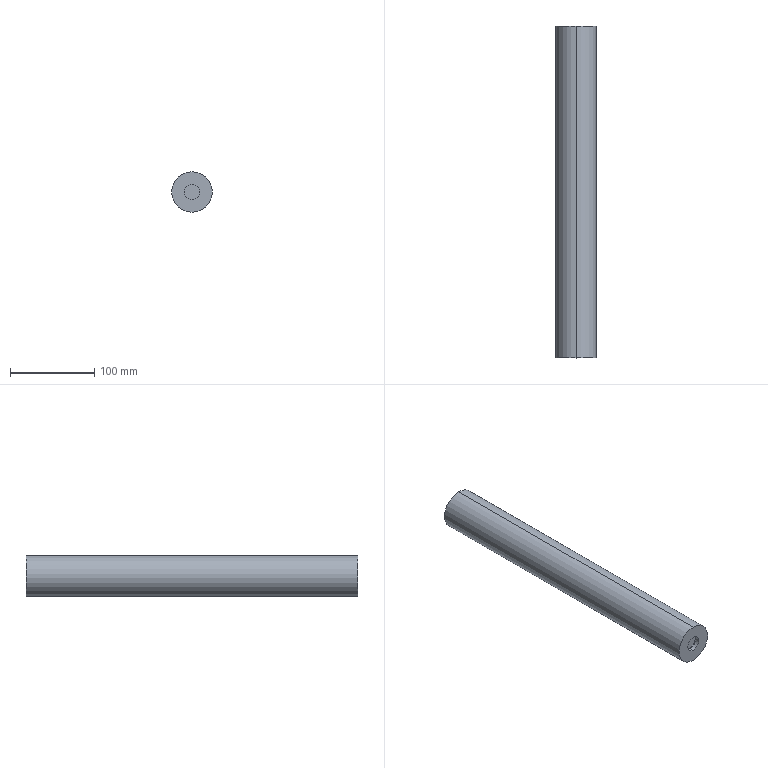Part | SolidWorks | features 3DProfileFeature 1, HoleWzd 1, Revolution 1 | 1 solid | 14 faces | box 48 x 395 x 48 mm | volume 696230 mm3 | cylinder 8 | plane 4 | cone 2 | commonest cylinder face diameters 18.5 x2 23 x2 25 x2 48 x2
STEP:
#1=CARTESIAN_POINT('',(0.,365.,-12.5));
#2=VERTEX_POINT('',#1);
#3=CARTESIAN_POINT('',(0.,365.,12.5));
#4=VERTEX_POINT('',#3);
#5=CARTESIAN_POINT('',(0.,365.,0.));
#6=DIRECTION('',(0.,1.,0.));
#7=DIRECTION('',(0.,0.,1.));
#8=AXIS2_PLACEMENT_3D('',#5,#6,#7);
#9=CIRCLE('',#8,12.5);
#10=EDGE_CURVE('',#2,#4,#9,.T.);
#11=ORIENTED_EDGE('',*,*,#10,.F.);
#12=CARTESIAN_POINT('',(0.,395.,-12.5));
#13=VERTEX_POINT('',#12);
#14=CARTESIAN_POINT('',(0.,395.,-12.5));
#15=DIRECTION('',(0.,1.,0.));
#16=VECTOR('',#15,1000.);
#17=LINE('',#14,#16);
#18=EDGE_CURVE('',#2,#13,#17,.T.);
#19=ORIENTED_EDGE('',*,*,#18,.T.);
#20=CARTESIAN_POINT('',(0.,395.,12.5));
#21=VERTEX_POINT('',#20);
#22=CARTESIAN_POINT('',(0.,395.,0.));
#23=DIRECTION('',(0.,1.,0.));
#24=DIRECTION('',(0.,0.,1.));
#25=AXIS2_PLACEMENT_3D('',#22,#23,#24);
#26=CIRCLE('',#25,12.5);
#27=EDGE_CURVE('',#13,#21,#26,.T.);
#28=ORIENTED_EDGE('',*,*,#27,.T.);
#29=CARTESIAN_POINT('',(0.,395.,12.5));
#30=DIRECTION('',(0.,1.,0.));
#31=VECTOR('',#30,1000.);
#32=LINE('',#29,#31);
#33=EDGE_CURVE('',#4,#21,#32,.T.);
#34=ORIENTED_EDGE('',*,*,#33,.F.);
#35=EDGE_LOOP('',(#11,#19,#28,#34));
#36=FACE_OUTER_BOUND('',#35,.T.);
#37=CARTESIAN_POINT('',(0.,395.,0.));
#38=DIRECTION('',(0.,1.,0.));
#39=DIRECTION('',(0.,0.,1.));
#40=AXIS2_PLACEMENT_3D('',#37,#38,#39);
#41=CYLINDRICAL_SURFACE('',#40,12.5);
#42=ADVANCED_FACE('',(#36),#41,.F.);
#43=CARTESIAN_POINT('',(0.,357.489,0.));
#44=VERTEX_POINT('',#43);
#45=CARTESIAN_POINT('',(0.,365.,12.5));
#46=DIRECTION('',(0.,0.515,0.8572));
#47=VECTOR('',#46,1000.);
#48=LINE('',#45,#47);
#49=EDGE_CURVE('',#44,#4,#48,.T.);
#50=ORIENTED_EDGE('',*,*,#49,.F.);
#51=CARTESIAN_POINT('',(0.,365.,-12.5));
#52=DIRECTION('',(0.,0.515,-0.8572));
#53=VECTOR('',#52,1000.);
#54=LINE('',#51,#53);
#55=EDGE_CURVE('',#44,#2,#54,.T.);
#56=ORIENTED_EDGE('',*,*,#55,.T.);
#57=ORIENTED_EDGE('',*,*,#10,.T.);
#58=EDGE_LOOP('',(#50,#56,#57));
#59=FACE_OUTER_BOUND('',#58,.T.);
#60=CARTESIAN_POINT('',(0.,365.,0.));
#61=DIRECTION('',(0.,1.,0.));
#62=DIRECTION('',(0.,0.,1.));
#63=AXIS2_PLACEMENT_3D('',#60,#61,#62);
#64=CONICAL_SURFACE('',#63,12.5,1.03);
#65=ADVANCED_FACE('',(#59),#64,.F.);
#66=CARTESIAN_POINT('',(0.,8.,11.5));
#67=VERTEX_POINT('',#66);
#68=CARTESIAN_POINT('',(0.,8.,-11.5));
#69=VERTEX_POINT('',#68);
#70=CARTESIAN_POINT('',(0.,8.,0.));
#71=DIRECTION('',(0.,-1.,0.));
#72=DIRECTION('',(0.,0.,-1.));
#73=AXIS2_PLACEMENT_3D('',#70,#71,#72);
#74=CIRCLE('',#73,11.5);
#75=EDGE_CURVE('',#67,#69,#74,.T.);
#76=ORIENTED_EDGE('',*,*,#75,.F.);
#77=CARTESIAN_POINT('',(0.,5.,11.5));
#78=VERTEX_POINT('',#77);
#79=CARTESIAN_POINT('',(0.,0.,11.5));
#80=DIRECTION('',(0.,-1.,0.));
#81=VECTOR('',#80,1000.);
#82=LINE('',#79,#81);
#83=EDGE_CURVE('',#67,#78,#82,.T.);
#84=ORIENTED_EDGE('',*,*,#83,.T.);
#85=CARTESIAN_POINT('',(0.,5.,-11.5));
#86=VERTEX_POINT('',#85);
#87=CARTESIAN_POINT('',(0.,5.,0.));
#88=DIRECTION('',(0.,-1.,0.));
#89=DIRECTION('',(0.,0.,-1.));
#90=AXIS2_PLACEMENT_3D('',#87,#88,#89);
#91=CIRCLE('',#90,11.5);
#92=EDGE_CURVE('',#78,#86,#91,.T.);
#93=ORIENTED_EDGE('',*,*,#92,.T.);
#94=CARTESIAN_POINT('',(0.,0.,-11.5));
#95=DIRECTION('',(0.,-1.,0.));
#96=VECTOR('',#95,1000.);
#97=LINE('',#94,#96);
#98=EDGE_CURVE('',#69,#86,#97,.T.);
#99=ORIENTED_EDGE('',*,*,#98,.F.);
#100=EDGE_LOOP('',(#76,#84,#93,#99));
#101=FACE_OUTER_BOUND('',#100,.T.);
#102=CARTESIAN_POINT('',(0.,0.,0.));
#103=DIRECTION('',(0.,-1.,0.));
#104=DIRECTION('',(0.,0.,-1.));
#105=AXIS2_PLACEMENT_3D('',#102,#103,#104);
#106=CYLINDRICAL_SURFACE('',#105,11.5);
#107=ADVANCED_FACE('',(#101),#106,.F.);
#108=CARTESIAN_POINT('',(0.,5.,9.25));
#109=VERTEX_POINT('',#108);
#110=CARTESIAN_POINT('',(0.,5.,-9.25));
#111=VERTEX_POINT('',#110);
#112=CARTESIAN_POINT('',(0.,5.,0.));
#113=DIRECTION('',(0.,-1.,0.));
#114=DIRECTION('',(0.,0.,-1.));
#115=AXIS2_PLACEMENT_3D('',#112,#113,#114);
#116=CIRCLE('',#115,9.25);
#117=EDGE_CURVE('',#109,#111,#116,.T.);
#118=ORIENTED_EDGE('',*,*,#117,.F.);
#119=CARTESIAN_POINT('',(0.,0.,9.25));
#120=VERTEX_POINT('',#119);
#121=CARTESIAN_POINT('',(0.,0.,9.25));
#122=DIRECTION('',(0.,-1.,0.));
#123=VECTOR('',#122,1000.);
#124=LINE('',#121,#123);
#125=EDGE_CURVE('',#109,#120,#124,.T.);
#126=ORIENTED_EDGE('',*,*,#125,.T.);
#127=CARTESIAN_POINT('',(0.,0.,-9.25));
#128=VERTEX_POINT('',#127);
#129=CARTESIAN_POINT('',(0.,0.,0.));
#130=DIRECTION('',(0.,-1.,0.));
#131=DIRECTION('',(0.,0.,-1.));
#132=AXIS2_PLACEMENT_3D('',#129,#130,#131);
#133=CIRCLE('',#132,9.25);
#134=EDGE_CURVE('',#120,#128,#133,.T.);
#135=ORIENTED_EDGE('',*,*,#134,.T.);
#136=CARTESIAN_POINT('',(0.,0.,-9.25));
#137=DIRECTION('',(0.,-1.,0.));
#138=VECTOR('',#137,1000.);
#139=LINE('',#136,#138);
#140=EDGE_CURVE('',#111,#128,#139,.T.);
#141=ORIENTED_EDGE('',*,*,#140,.F.);
#142=EDGE_LOOP('',(#118,#126,#135,#141));
#143=FACE_OUTER_BOUND('',#142,.T.);
#144=CARTESIAN_POINT('',(0.,0.,0.));
#145=DIRECTION('',(0.,-1.,0.));
#146=DIRECTION('',(0.,0.,-1.));
#147=AXIS2_PLACEMENT_3D('',#144,#145,#146);
#148=CYLINDRICAL_SURFACE('',#147,9.25);
#149=ADVANCED_FACE('',(#143),#148,.F.);
#150=CARTESIAN_POINT('',(0.,395.,-24.));
#151=VERTEX_POINT('',#150);
#152=CARTESIAN_POINT('',(0.,395.,24.));
#153=VERTEX_POINT('',#152);
#154=CARTESIAN_POINT('',(0.,395.,0.));
#155=DIRECTION('',(0.,-1.,0.));
#156=DIRECTION('',(0.,0.,-1.));
#157=AXIS2_PLACEMENT_3D('',#154,#155,#156);
#158=CIRCLE('',#157,24.);
#159=EDGE_CURVE('',#151,#153,#158,.T.);
#160=ORIENTED_EDGE('',*,*,#159,.T.);
#161=CARTESIAN_POINT('',(0.,0.,24.));
#162=VERTEX_POINT('',#161);
#163=CARTESIAN_POINT('',(0.,0.,24.));
#164=DIRECTION('',(0.,-1.,0.));
#165=VECTOR('',#164,1000.);
#166=LINE('',#163,#165);
#167=EDGE_CURVE('',#153,#162,#166,.T.);
#168=ORIENTED_EDGE('',*,*,#167,.T.);
#169=CARTESIAN_POINT('',(0.,0.,-24.));
#170=VERTEX_POINT('',#169);
#171=CARTESIAN_POINT('',(0.,0.,0.));
#172=DIRECTION('',(0.,-1.,0.));
#173=DIRECTION('',(0.,0.,-1.));
#174=AXIS2_PLACEMENT_3D('',#171,#172,#173);
#175=CIRCLE('',#174,24.);
#176=EDGE_CURVE('',#170,#162,#175,.T.);
#177=ORIENTED_EDGE('',*,*,#176,.F.);
#178=CARTESIAN_POINT('',(0.,0.,-24.));
#179=DIRECTION('',(0.,-1.,0.));
#180=VECTOR('',#179,1000.);
#181=LINE('',#178,#180);
#182=EDGE_CURVE('',#151,#170,#181,.T.);
#183=ORIENTED_EDGE('',*,*,#182,.F.);
#184=EDGE_LOOP('',(#160,#168,#177,#183));
#185=FACE_OUTER_BOUND('',#184,.T.);
#186=CARTESIAN_POINT('',(0.,0.,0.));
#187=DIRECTION('',(0.,-1.,0.));
#188=DIRECTION('',(0.,0.,-1.));
#189=AXIS2_PLACEMENT_3D('',#186,#187,#188);
#190=CYLINDRICAL_SURFACE('',#189,24.);
#191=ADVANCED_FACE('',(#185),#190,.T.);
#192=CARTESIAN_POINT('',(0.,395.,0.));
#193=DIRECTION('',(0.,1.,0.));
#194=DIRECTION('',(0.,0.,1.));
#195=AXIS2_PLACEMENT_3D('',#192,#193,#194);
#196=CIRCLE('',#195,12.5);
#197=EDGE_CURVE('',#21,#13,#196,.T.);
#198=ORIENTED_EDGE('',*,*,#197,.F.);
#199=ORIENTED_EDGE('',*,*,#27,.F.);
#200=EDGE_LOOP('',(#198,#199));
#201=FACE_BOUND('',#200,.T.);
#202=ORIENTED_EDGE('',*,*,#159,.F.);
#203=CARTESIAN_POINT('',(0.,395.,0.));
#204=DIRECTION('',(0.,-1.,0.));
#205=DIRECTION('',(0.,0.,-1.));
#206=AXIS2_PLACEMENT_3D('',#203,#204,#205);
#207=CIRCLE('',#206,24.);
#208=EDGE_CURVE('',#153,#151,#207,.T.);
#209=ORIENTED_EDGE('',*,*,#208,.F.);
#210=EDGE_LOOP('',(#202,#209));
#211=FACE_OUTER_BOUND('',#210,.T.);
#212=CARTESIAN_POINT('',(0.,395.,0.));
#213=DIRECTION('',(0.,1.,0.));
#214=DIRECTION('',(0.,0.,1.));
#215=AXIS2_PLACEMENT_3D('',#212,#213,#214);
#216=PLANE('',#215);
#217=ADVANCED_FACE('',(#201,#211),#216,.T.);
#218=ORIENTED_EDGE('',*,*,#167,.F.);
#219=ORIENTED_EDGE('',*,*,#208,.T.);
#220=ORIENTED_EDGE('',*,*,#182,.T.);
#221=CARTESIAN_POINT('',(0.,0.,0.));
#222=DIRECTION('',(0.,-1.,0.));
#223=DIRECTION('',(0.,0.,-1.));
#224=AXIS2_PLACEMENT_3D('',#221,#222,#223);
#225=CIRCLE('',#224,24.);
#226=EDGE_CURVE('',#162,#170,#225,.T.);
#227=ORIENTED_EDGE('',*,*,#226,.F.);
#228=EDGE_LOOP('',(#218,#219,#220,#227));
#229=FACE_OUTER_BOUND('',#228,.T.);
#230=CARTESIAN_POINT('',(0.,0.,0.));
#231=DIRECTION('',(0.,-1.,0.));
#232=DIRECTION('',(0.,0.,-1.));
#233=AXIS2_PLACEMENT_3D('',#230,#231,#232);
#234=CYLINDRICAL_SURFACE('',#233,24.);
#235=ADVANCED_FACE('',(#229),#234,.T.);
#236=ORIENTED_EDGE('',*,*,#176,.T.);
#237=ORIENTED_EDGE('',*,*,#226,.T.);
#238=EDGE_LOOP('',(#236,#237));
#239=FACE_OUTER_BOUND('',#238,.T.);
#240=CARTESIAN_POINT('',(0.,0.,0.));
#241=DIRECTION('',(0.,-1.,0.));
#242=DIRECTION('',(0.,0.,-1.));
#243=AXIS2_PLACEMENT_3D('',#240,#241,#242);
#244=CIRCLE('',#243,9.25);
#245=EDGE_CURVE('',#128,#120,#244,.T.);
#246=ORIENTED_EDGE('',*,*,#245,.F.);
#247=ORIENTED_EDGE('',*,*,#134,.F.);
#248=EDGE_LOOP('',(#246,#247));
#249=FACE_BOUND('',#248,.T.);
#250=CARTESIAN_POINT('',(0.,0.,-24.));
#251=DIRECTION('',(0.,-1.,0.));
#252=DIRECTION('',(0.,0.,-1.));
#253=AXIS2_PLACEMENT_3D('',#250,#251,#252);
#254=PLANE('',#253);
#255=ADVANCED_FACE('',(#239,#249),#254,.T.);
#256=ORIENTED_EDGE('',*,*,#125,.F.);
#257=CARTESIAN_POINT('',(0.,5.,0.));
#258=DIRECTION('',(0.,-1.,0.));
#259=DIRECTION('',(0.,0.,-1.));
#260=AXIS2_PLACEMENT_3D('',#257,#258,#259);
#261=CIRCLE('',#260,9.25);
#262=EDGE_CURVE('',#111,#109,#261,.T.);
#263=ORIENTED_EDGE('',*,*,#262,.F.);
#264=ORIENTED_EDGE('',*,*,#140,.T.);
#265=ORIENTED_EDGE('',*,*,#245,.T.);
#266=EDGE_LOOP('',(#256,#263,#264,#265));
#267=FACE_OUTER_BOUND('',#266,.T.);
#268=CARTESIAN_POINT('',(0.,0.,0.));
#269=DIRECTION('',(0.,-1.,0.));
#270=DIRECTION('',(0.,0.,-1.));
#271=AXIS2_PLACEMENT_3D('',#268,#269,#270);
#272=CYLINDRICAL_SURFACE('',#271,9.25);
#273=ADVANCED_FACE('',(#267),#272,.F.);
#274=ORIENTED_EDGE('',*,*,#262,.T.);
#275=ORIENTED_EDGE('',*,*,#117,.T.);
#276=EDGE_LOOP('',(#274,#275));
#277=FACE_BOUND('',#276,.T.);
#278=CARTESIAN_POINT('',(0.,5.,0.));
#279=DIRECTION('',(0.,-1.,0.));
#280=DIRECTION('',(0.,0.,-1.));
#281=AXIS2_PLACEMENT_3D('',#278,#279,#280);
#282=CIRCLE('',#281,11.5);
#283=EDGE_CURVE('',#86,#78,#282,.T.);
#284=ORIENTED_EDGE('',*,*,#283,.F.);
#285=ORIENTED_EDGE('',*,*,#92,.F.);
#286=EDGE_LOOP('',(#284,#285));
#287=FACE_OUTER_BOUND('',#286,.T.);
#288=CARTESIAN_POINT('',(0.,5.,-9.25));
#289=DIRECTION('',(0.,1.,0.));
#290=DIRECTION('',(0.,0.,1.));
#291=AXIS2_PLACEMENT_3D('',#288,#289,#290);
#292=PLANE('',#291);
#293=ADVANCED_FACE('',(#277,#287),#292,.T.);
#294=ORIENTED_EDGE('',*,*,#83,.F.);
#295=CARTESIAN_POINT('',(0.,8.,0.));
#296=DIRECTION('',(0.,-1.,0.));
#297=DIRECTION('',(0.,0.,-1.));
#298=AXIS2_PLACEMENT_3D('',#295,#296,#297);
#299=CIRCLE('',#298,11.5);
#300=EDGE_CURVE('',#69,#67,#299,.T.);
#301=ORIENTED_EDGE('',*,*,#300,.F.);
#302=ORIENTED_EDGE('',*,*,#98,.T.);
#303=ORIENTED_EDGE('',*,*,#283,.T.);
#304=EDGE_LOOP('',(#294,#301,#302,#303));
#305=FACE_OUTER_BOUND('',#304,.T.);
#306=CARTESIAN_POINT('',(0.,0.,0.));
#307=DIRECTION('',(0.,-1.,0.));
#308=DIRECTION('',(0.,0.,-1.));
#309=AXIS2_PLACEMENT_3D('',#306,#307,#308);
#310=CYLINDRICAL_SURFACE('',#309,11.5);
#311=ADVANCED_FACE('',(#305),#310,.F.);
#312=ORIENTED_EDGE('',*,*,#300,.T.);
#313=ORIENTED_EDGE('',*,*,#75,.T.);
#314=EDGE_LOOP('',(#312,#313));
#315=FACE_OUTER_BOUND('',#314,.T.);
#316=CARTESIAN_POINT('',(0.,8.,-11.5));
#317=DIRECTION('',(0.,-1.,0.));
#318=DIRECTION('',(0.,0.,-1.));
#319=AXIS2_PLACEMENT_3D('',#316,#317,#318);
#320=PLANE('',#319);
#321=ADVANCED_FACE('',(#315),#320,.T.);
#322=ORIENTED_EDGE('',*,*,#55,.F.);
#323=ORIENTED_EDGE('',*,*,#49,.T.);
#324=CARTESIAN_POINT('',(0.,365.,0.));
#325=DIRECTION('',(0.,1.,0.));
#326=DIRECTION('',(0.,0.,1.));
#327=AXIS2_PLACEMENT_3D('',#324,#325,#326);
#328=CIRCLE('',#327,12.5);
#329=EDGE_CURVE('',#4,#2,#328,.T.);
#330=ORIENTED_EDGE('',*,*,#329,.T.);
#331=EDGE_LOOP('',(#322,#323,#330));
#332=FACE_OUTER_BOUND('',#331,.T.);
#333=CARTESIAN_POINT('',(0.,365.,0.));
#334=DIRECTION('',(0.,1.,0.));
#335=DIRECTION('',(0.,0.,1.));
#336=AXIS2_PLACEMENT_3D('',#333,#334,#335);
#337=CONICAL_SURFACE('',#336,12.5,1.03);
#338=ADVANCED_FACE('',(#332),#337,.F.);
#339=ORIENTED_EDGE('',*,*,#18,.F.);
#340=ORIENTED_EDGE('',*,*,#329,.F.);
#341=ORIENTED_EDGE('',*,*,#33,.T.);
#342=ORIENTED_EDGE('',*,*,#197,.T.);
#343=EDGE_LOOP('',(#339,#340,#341,#342));
#344=FACE_OUTER_BOUND('',#343,.T.);
#345=CARTESIAN_POINT('',(0.,395.,0.));
#346=DIRECTION('',(0.,1.,0.));
#347=DIRECTION('',(0.,0.,1.));
#348=AXIS2_PLACEMENT_3D('',#345,#346,#347);
#349=CYLINDRICAL_SURFACE('',#348,12.5);
#350=ADVANCED_FACE('',(#344),#349,.F.);
#351=CLOSED_SHELL('',(#42,#65,#107,#149,#191,#217,#235,#255,#273,#293,#311,#321,#338,#350));
#352=MANIFOLD_SOLID_BREP('',#351);
#353=CARTESIAN_POINT('',(0.,0.,0.));
#354=DIRECTION('',(0.,0.,1.));
#355=DIRECTION('',(1.,0.,0.));
#356=AXIS2_PLACEMENT_3D('',#353,#354,#355);
#357=(LENGTH_UNIT()NAMED_UNIT(*)SI_UNIT(.MILLI.,.METRE.));
#358=UNCERTAINTY_MEASURE_WITH_UNIT(LENGTH_MEASURE(0.00001),#357,'','');
#359=(NAMED_UNIT(*)PLANE_ANGLE_UNIT()SI_UNIT($,.RADIAN.));
#360=(NAMED_UNIT(*)SI_UNIT($,.STERADIAN.)SOLID_ANGLE_UNIT());
#361=(GEOMETRIC_REPRESENTATION_CONTEXT(3)GLOBAL_UNCERTAINTY_ASSIGNED_CONTEXT((#358))GLOBAL_UNIT_ASSIGNED_CONTEXT((#357,#359,#360))REPRESENTATION_CONTEXT('',''));
#362=ADVANCED_BREP_SHAPE_REPRESENTATION('',(#352,#356),#361);